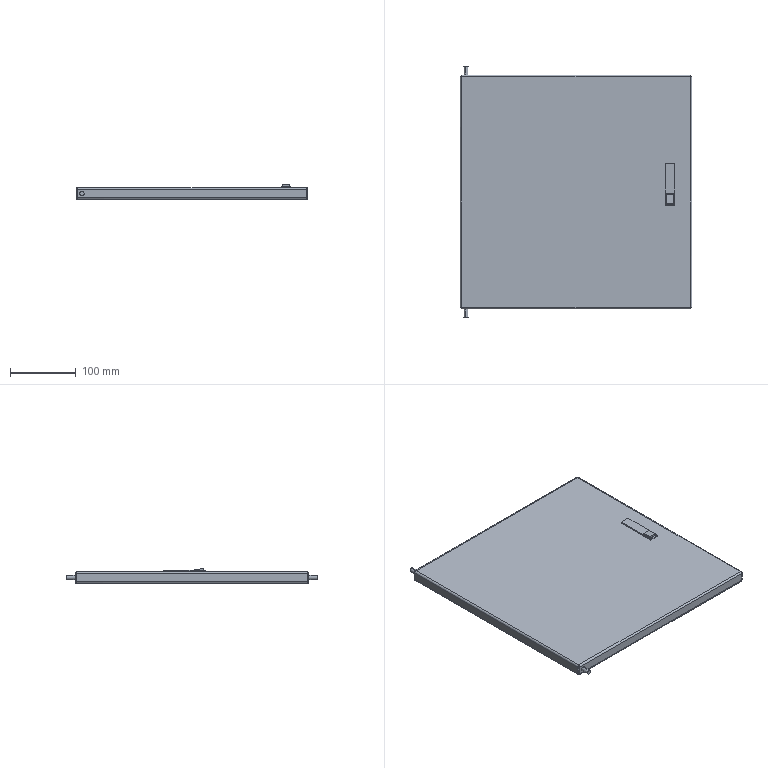Part | STEP file | panel body depan | 4 solids | 108 faces | box 352 x 381.4 x 22.754 mm | volume 281354 mm3 | plane 68 | cylinder 24 | spline 16 | commonest cylinder face diameters 2 x8 5.6 x8 6.5 x4 6.6 x4